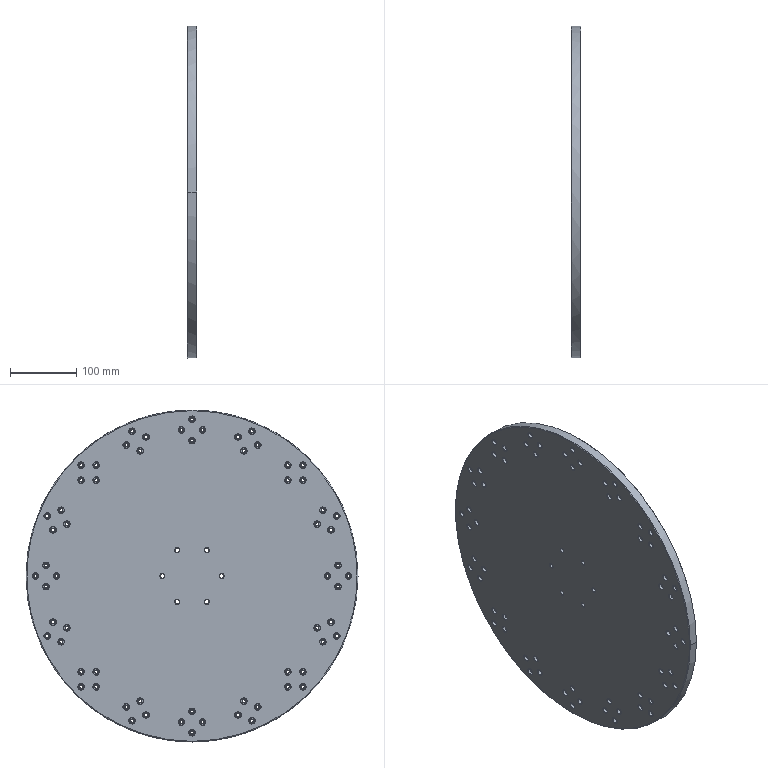Part | STEP file | 05-01 Turntable | 1 solid | 776 faces | box 15 x 500 x 500 mm | volume 2906258 mm3 | cone 422 | cylinder 282 | plane 72 | commonest cylinder face diameters 4.5 x128 9 x128 6.5 x12 12 x12 500 x2